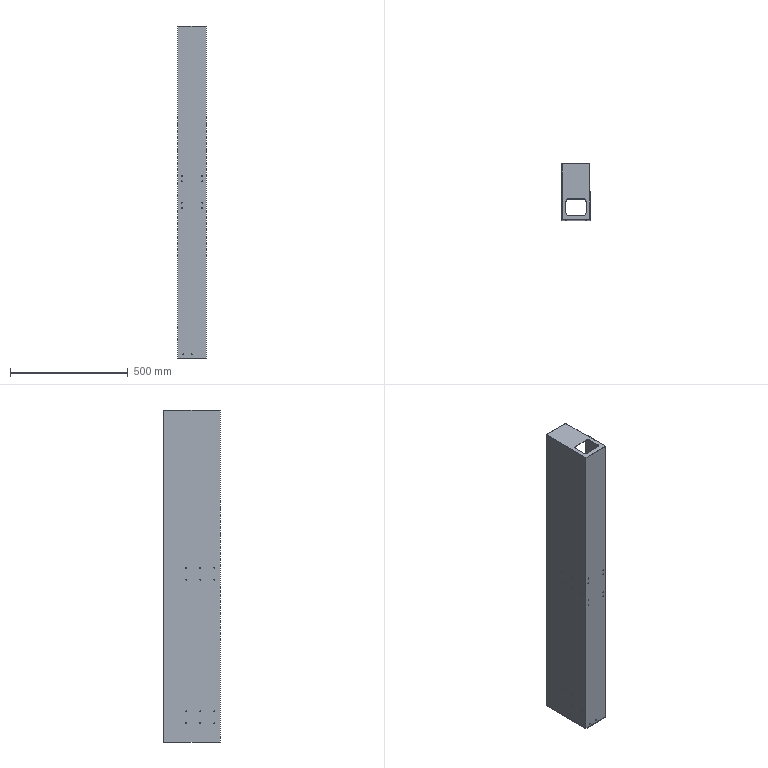Part | NX | 1 solid | 64 faces | box 120 x 240 x 1410 mm | volume 1454047 mm3 | cylinder 38 | plane 26 | commonest cylinder face diameters 4.2 x22 2.5 x8 20 x8